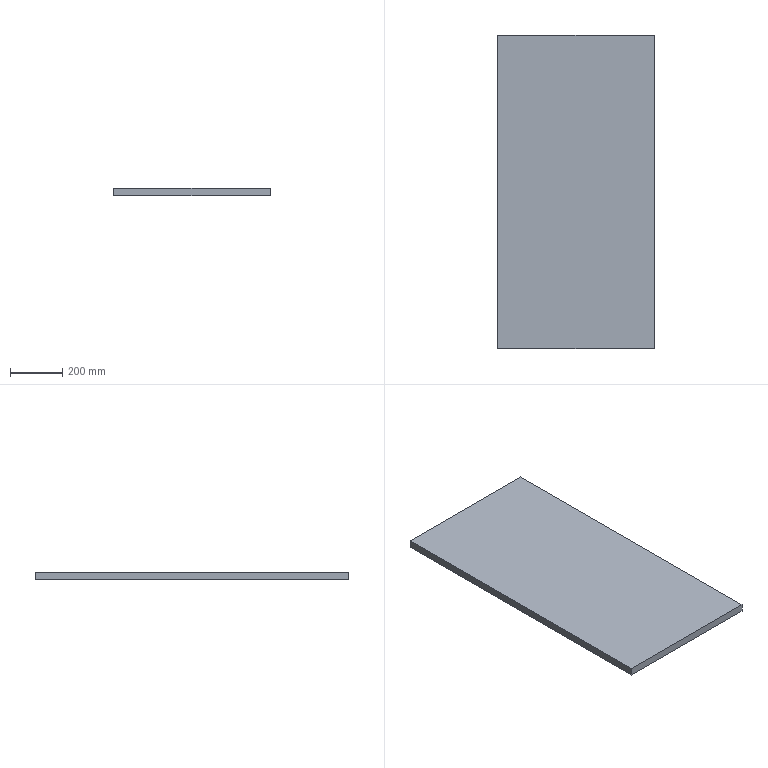Part | SolidWorks | features Extrusion 1, ICE 1 | 1 solid | 18 faces | box 600 x 1200 x 30 mm | volume 21509522 mm3 | plane 10 | cylinder 8 | commonest cylinder face diameters 120 x8
STEP:
#1=CARTESIAN_POINT('',(240.,-480.,2.));
#2=VERTEX_POINT('',#1);
#3=CARTESIAN_POINT('',(120.,-480.,2.));
#4=VERTEX_POINT('',#3);
#5=CARTESIAN_POINT('',(180.,-480.,2.));
#6=DIRECTION('',(0.,0.,-1.));
#7=DIRECTION('',(1.,0.,0.));
#8=AXIS2_PLACEMENT_3D('',#5,#6,#7);
#9=CIRCLE('',#8,60.);
#10=EDGE_CURVE('',#2,#4,#9,.T.);
#11=ORIENTED_EDGE('',*,*,#10,.F.);
#12=CARTESIAN_POINT('',(240.,-480.,0.));
#13=VERTEX_POINT('',#12);
#14=CARTESIAN_POINT('',(240.,-480.,2.));
#15=DIRECTION('',(0.,0.,-1.));
#16=VECTOR('',#15,1000.);
#17=LINE('',#14,#16);
#18=EDGE_CURVE('',#2,#13,#17,.T.);
#19=ORIENTED_EDGE('',*,*,#18,.T.);
#20=CARTESIAN_POINT('',(120.,-480.,0.));
#21=VERTEX_POINT('',#20);
#22=CARTESIAN_POINT('',(180.,-480.,0.));
#23=DIRECTION('',(0.,0.,-1.));
#24=DIRECTION('',(1.,0.,0.));
#25=AXIS2_PLACEMENT_3D('',#22,#23,#24);
#26=CIRCLE('',#25,60.);
#27=EDGE_CURVE('',#13,#21,#26,.T.);
#28=ORIENTED_EDGE('',*,*,#27,.T.);
#29=CARTESIAN_POINT('',(120.,-480.,2.));
#30=DIRECTION('',(0.,0.,-1.));
#31=VECTOR('',#30,1000.);
#32=LINE('',#29,#31);
#33=EDGE_CURVE('',#4,#21,#32,.T.);
#34=ORIENTED_EDGE('',*,*,#33,.F.);
#35=EDGE_LOOP('',(#11,#19,#28,#34));
#36=FACE_OUTER_BOUND('',#35,.T.);
#37=CARTESIAN_POINT('',(180.,-480.,2.));
#38=DIRECTION('',(0.,0.,-1.));
#39=DIRECTION('',(-1.,0.,0.));
#40=AXIS2_PLACEMENT_3D('',#37,#38,#39);
#41=CYLINDRICAL_SURFACE('',#40,60.);
#42=ADVANCED_FACE('',(#36),#41,.F.);
#43=CARTESIAN_POINT('',(-120.,-480.,2.));
#44=VERTEX_POINT('',#43);
#45=CARTESIAN_POINT('',(-240.,-480.,2.));
#46=VERTEX_POINT('',#45);
#47=CARTESIAN_POINT('',(-180.,-480.,2.));
#48=DIRECTION('',(0.,0.,-1.));
#49=DIRECTION('',(-1.,0.,0.));
#50=AXIS2_PLACEMENT_3D('',#47,#48,#49);
#51=CIRCLE('',#50,60.);
#52=EDGE_CURVE('',#44,#46,#51,.T.);
#53=ORIENTED_EDGE('',*,*,#52,.F.);
#54=CARTESIAN_POINT('',(-120.,-480.,0.));
#55=VERTEX_POINT('',#54);
#56=CARTESIAN_POINT('',(-120.,-480.,2.));
#57=DIRECTION('',(0.,0.,-1.));
#58=VECTOR('',#57,1000.);
#59=LINE('',#56,#58);
#60=EDGE_CURVE('',#44,#55,#59,.T.);
#61=ORIENTED_EDGE('',*,*,#60,.T.);
#62=CARTESIAN_POINT('',(-240.,-480.,0.));
#63=VERTEX_POINT('',#62);
#64=CARTESIAN_POINT('',(-180.,-480.,0.));
#65=DIRECTION('',(0.,0.,-1.));
#66=DIRECTION('',(-1.,0.,0.));
#67=AXIS2_PLACEMENT_3D('',#64,#65,#66);
#68=CIRCLE('',#67,60.);
#69=EDGE_CURVE('',#55,#63,#68,.T.);
#70=ORIENTED_EDGE('',*,*,#69,.T.);
#71=CARTESIAN_POINT('',(-240.,-480.,2.));
#72=DIRECTION('',(0.,0.,-1.));
#73=VECTOR('',#72,1000.);
#74=LINE('',#71,#73);
#75=EDGE_CURVE('',#46,#63,#74,.T.);
#76=ORIENTED_EDGE('',*,*,#75,.F.);
#77=EDGE_LOOP('',(#53,#61,#70,#76));
#78=FACE_OUTER_BOUND('',#77,.T.);
#79=CARTESIAN_POINT('',(-180.,-480.,2.));
#80=DIRECTION('',(0.,0.,-1.));
#81=DIRECTION('',(-1.,0.,0.));
#82=AXIS2_PLACEMENT_3D('',#79,#80,#81);
#83=CYLINDRICAL_SURFACE('',#82,60.);
#84=ADVANCED_FACE('',(#78),#83,.F.);
#85=CARTESIAN_POINT('',(-120.,480.,2.));
#86=VERTEX_POINT('',#85);
#87=CARTESIAN_POINT('',(-240.,480.,2.));
#88=VERTEX_POINT('',#87);
#89=CARTESIAN_POINT('',(-180.,480.,2.));
#90=DIRECTION('',(0.,0.,-1.));
#91=DIRECTION('',(1.,0.,0.));
#92=AXIS2_PLACEMENT_3D('',#89,#90,#91);
#93=CIRCLE('',#92,60.);
#94=EDGE_CURVE('',#86,#88,#93,.T.);
#95=ORIENTED_EDGE('',*,*,#94,.F.);
#96=CARTESIAN_POINT('',(-120.,480.,0.));
#97=VERTEX_POINT('',#96);
#98=CARTESIAN_POINT('',(-120.,480.,2.));
#99=DIRECTION('',(0.,0.,-1.));
#100=VECTOR('',#99,1000.);
#101=LINE('',#98,#100);
#102=EDGE_CURVE('',#86,#97,#101,.T.);
#103=ORIENTED_EDGE('',*,*,#102,.T.);
#104=CARTESIAN_POINT('',(-240.,480.,0.));
#105=VERTEX_POINT('',#104);
#106=CARTESIAN_POINT('',(-180.,480.,0.));
#107=DIRECTION('',(0.,0.,-1.));
#108=DIRECTION('',(1.,0.,0.));
#109=AXIS2_PLACEMENT_3D('',#106,#107,#108);
#110=CIRCLE('',#109,60.);
#111=EDGE_CURVE('',#97,#105,#110,.T.);
#112=ORIENTED_EDGE('',*,*,#111,.T.);
#113=CARTESIAN_POINT('',(-240.,480.,2.));
#114=DIRECTION('',(0.,0.,-1.));
#115=VECTOR('',#114,1000.);
#116=LINE('',#113,#115);
#117=EDGE_CURVE('',#88,#105,#116,.T.);
#118=ORIENTED_EDGE('',*,*,#117,.F.);
#119=EDGE_LOOP('',(#95,#103,#112,#118));
#120=FACE_OUTER_BOUND('',#119,.T.);
#121=CARTESIAN_POINT('',(-180.,480.,2.));
#122=DIRECTION('',(0.,0.,-1.));
#123=DIRECTION('',(-1.,0.,0.));
#124=AXIS2_PLACEMENT_3D('',#121,#122,#123);
#125=CYLINDRICAL_SURFACE('',#124,60.);
#126=ADVANCED_FACE('',(#120),#125,.F.);
#127=CARTESIAN_POINT('',(240.,480.,2.));
#128=VERTEX_POINT('',#127);
#129=CARTESIAN_POINT('',(120.,480.,2.));
#130=VERTEX_POINT('',#129);
#131=CARTESIAN_POINT('',(180.,480.,2.));
#132=DIRECTION('',(0.,0.,-1.));
#133=DIRECTION('',(-1.,0.,0.));
#134=AXIS2_PLACEMENT_3D('',#131,#132,#133);
#135=CIRCLE('',#134,60.);
#136=EDGE_CURVE('',#128,#130,#135,.T.);
#137=ORIENTED_EDGE('',*,*,#136,.F.);
#138=CARTESIAN_POINT('',(240.,480.,0.));
#139=VERTEX_POINT('',#138);
#140=CARTESIAN_POINT('',(240.,480.,2.));
#141=DIRECTION('',(0.,0.,-1.));
#142=VECTOR('',#141,1000.);
#143=LINE('',#140,#142);
#144=EDGE_CURVE('',#128,#139,#143,.T.);
#145=ORIENTED_EDGE('',*,*,#144,.T.);
#146=CARTESIAN_POINT('',(120.,480.,0.));
#147=VERTEX_POINT('',#146);
#148=CARTESIAN_POINT('',(180.,480.,0.));
#149=DIRECTION('',(0.,0.,-1.));
#150=DIRECTION('',(-1.,0.,0.));
#151=AXIS2_PLACEMENT_3D('',#148,#149,#150);
#152=CIRCLE('',#151,60.);
#153=EDGE_CURVE('',#139,#147,#152,.T.);
#154=ORIENTED_EDGE('',*,*,#153,.T.);
#155=CARTESIAN_POINT('',(120.,480.,2.));
#156=DIRECTION('',(0.,0.,-1.));
#157=VECTOR('',#156,1000.);
#158=LINE('',#155,#157);
#159=EDGE_CURVE('',#130,#147,#158,.T.);
#160=ORIENTED_EDGE('',*,*,#159,.F.);
#161=EDGE_LOOP('',(#137,#145,#154,#160));
#162=FACE_OUTER_BOUND('',#161,.T.);
#163=CARTESIAN_POINT('',(180.,480.,2.));
#164=DIRECTION('',(0.,0.,-1.));
#165=DIRECTION('',(-1.,0.,0.));
#166=AXIS2_PLACEMENT_3D('',#163,#164,#165);
#167=CYLINDRICAL_SURFACE('',#166,60.);
#168=ADVANCED_FACE('',(#162),#167,.F.);
#169=CARTESIAN_POINT('',(300.,-600.,0.));
#170=VERTEX_POINT('',#169);
#171=CARTESIAN_POINT('',(300.,600.,0.));
#172=VERTEX_POINT('',#171);
#173=CARTESIAN_POINT('',(300.,-600.,0.));
#174=DIRECTION('',(0.,1.,0.));
#175=VECTOR('',#174,1000.);
#176=LINE('',#173,#175);
#177=EDGE_CURVE('',#170,#172,#176,.T.);
#178=ORIENTED_EDGE('',*,*,#177,.T.);
#179=CARTESIAN_POINT('',(300.,600.,30.));
#180=VERTEX_POINT('',#179);
#181=CARTESIAN_POINT('',(300.,600.,30.));
#182=DIRECTION('',(0.,0.,-1.));
#183=VECTOR('',#182,1000.);
#184=LINE('',#181,#183);
#185=EDGE_CURVE('',#180,#172,#184,.T.);
#186=ORIENTED_EDGE('',*,*,#185,.F.);
#187=CARTESIAN_POINT('',(300.,-600.,30.));
#188=VERTEX_POINT('',#187);
#189=CARTESIAN_POINT('',(300.,-600.,30.));
#190=DIRECTION('',(0.,1.,0.));
#191=VECTOR('',#190,1000.);
#192=LINE('',#189,#191);
#193=EDGE_CURVE('',#188,#180,#192,.T.);
#194=ORIENTED_EDGE('',*,*,#193,.F.);
#195=CARTESIAN_POINT('',(300.,-600.,30.));
#196=DIRECTION('',(0.,0.,-1.));
#197=VECTOR('',#196,1000.);
#198=LINE('',#195,#197);
#199=EDGE_CURVE('',#188,#170,#198,.T.);
#200=ORIENTED_EDGE('',*,*,#199,.T.);
#201=EDGE_LOOP('',(#178,#186,#194,#200));
#202=FACE_OUTER_BOUND('',#201,.T.);
#203=CARTESIAN_POINT('',(300.,-600.,30.));
#204=DIRECTION('',(-1.,0.,0.));
#205=DIRECTION('',(0.,0.,1.));
#206=AXIS2_PLACEMENT_3D('',#203,#204,#205);
#207=PLANE('',#206);
#208=ADVANCED_FACE('',(#202),#207,.F.);
#209=CARTESIAN_POINT('',(-300.,600.,0.));
#210=VERTEX_POINT('',#209);
#211=CARTESIAN_POINT('',(-300.,600.,0.));
#212=DIRECTION('',(-1.,0.,0.));
#213=VECTOR('',#212,1000.);
#214=LINE('',#211,#213);
#215=EDGE_CURVE('',#172,#210,#214,.T.);
#216=ORIENTED_EDGE('',*,*,#215,.T.);
#217=CARTESIAN_POINT('',(-300.,600.,30.));
#218=VERTEX_POINT('',#217);
#219=CARTESIAN_POINT('',(-300.,600.,30.));
#220=DIRECTION('',(0.,0.,-1.));
#221=VECTOR('',#220,1000.);
#222=LINE('',#219,#221);
#223=EDGE_CURVE('',#218,#210,#222,.T.);
#224=ORIENTED_EDGE('',*,*,#223,.F.);
#225=CARTESIAN_POINT('',(-300.,600.,30.));
#226=DIRECTION('',(-1.,0.,0.));
#227=VECTOR('',#226,1000.);
#228=LINE('',#225,#227);
#229=EDGE_CURVE('',#180,#218,#228,.T.);
#230=ORIENTED_EDGE('',*,*,#229,.F.);
#231=ORIENTED_EDGE('',*,*,#185,.T.);
#232=EDGE_LOOP('',(#216,#224,#230,#231));
#233=FACE_OUTER_BOUND('',#232,.T.);
#234=CARTESIAN_POINT('',(-300.,600.,30.));
#235=DIRECTION('',(0.,-1.,0.));
#236=DIRECTION('',(0.,0.,-1.));
#237=AXIS2_PLACEMENT_3D('',#234,#235,#236);
#238=PLANE('',#237);
#239=ADVANCED_FACE('',(#233),#238,.F.);
#240=CARTESIAN_POINT('',(-300.,-600.,0.));
#241=VERTEX_POINT('',#240);
#242=CARTESIAN_POINT('',(-300.,-600.,0.));
#243=DIRECTION('',(0.,-1.,0.));
#244=VECTOR('',#243,1000.);
#245=LINE('',#242,#244);
#246=EDGE_CURVE('',#210,#241,#245,.T.);
#247=ORIENTED_EDGE('',*,*,#246,.T.);
#248=CARTESIAN_POINT('',(-300.,-600.,30.));
#249=VERTEX_POINT('',#248);
#250=CARTESIAN_POINT('',(-300.,-600.,30.));
#251=DIRECTION('',(0.,0.,-1.));
#252=VECTOR('',#251,1000.);
#253=LINE('',#250,#252);
#254=EDGE_CURVE('',#249,#241,#253,.T.);
#255=ORIENTED_EDGE('',*,*,#254,.F.);
#256=CARTESIAN_POINT('',(-300.,-600.,30.));
#257=DIRECTION('',(0.,-1.,0.));
#258=VECTOR('',#257,1000.);
#259=LINE('',#256,#258);
#260=EDGE_CURVE('',#218,#249,#259,.T.);
#261=ORIENTED_EDGE('',*,*,#260,.F.);
#262=ORIENTED_EDGE('',*,*,#223,.T.);
#263=EDGE_LOOP('',(#247,#255,#261,#262));
#264=FACE_OUTER_BOUND('',#263,.T.);
#265=CARTESIAN_POINT('',(-300.,-600.,30.));
#266=DIRECTION('',(1.,0.,0.));
#267=DIRECTION('',(0.,0.,-1.));
#268=AXIS2_PLACEMENT_3D('',#265,#266,#267);
#269=PLANE('',#268);
#270=ADVANCED_FACE('',(#264),#269,.F.);
#271=CARTESIAN_POINT('',(-300.,-600.,0.));
#272=DIRECTION('',(1.,0.,0.));
#273=VECTOR('',#272,1000.);
#274=LINE('',#271,#273);
#275=EDGE_CURVE('',#241,#170,#274,.T.);
#276=ORIENTED_EDGE('',*,*,#275,.T.);
#277=ORIENTED_EDGE('',*,*,#199,.F.);
#278=CARTESIAN_POINT('',(-300.,-600.,30.));
#279=DIRECTION('',(1.,0.,0.));
#280=VECTOR('',#279,1000.);
#281=LINE('',#278,#280);
#282=EDGE_CURVE('',#249,#188,#281,.T.);
#283=ORIENTED_EDGE('',*,*,#282,.F.);
#284=ORIENTED_EDGE('',*,*,#254,.T.);
#285=EDGE_LOOP('',(#276,#277,#283,#284));
#286=FACE_OUTER_BOUND('',#285,.T.);
#287=CARTESIAN_POINT('',(-300.,-600.,30.));
#288=DIRECTION('',(0.,1.,0.));
#289=DIRECTION('',(0.,0.,1.));
#290=AXIS2_PLACEMENT_3D('',#287,#288,#289);
#291=PLANE('',#290);
#292=ADVANCED_FACE('',(#286),#291,.F.);
#293=ORIENTED_EDGE('',*,*,#193,.T.);
#294=ORIENTED_EDGE('',*,*,#229,.T.);
#295=ORIENTED_EDGE('',*,*,#260,.T.);
#296=ORIENTED_EDGE('',*,*,#282,.T.);
#297=EDGE_LOOP('',(#293,#294,#295,#296));
#298=FACE_OUTER_BOUND('',#297,.T.);
#299=CARTESIAN_POINT('',(0.,0.,30.));
#300=DIRECTION('',(0.,0.,-1.));
#301=DIRECTION('',(-1.,0.,0.));
#302=AXIS2_PLACEMENT_3D('',#299,#300,#301);
#303=PLANE('',#302);
#304=ADVANCED_FACE('',(#298),#303,.F.);
#305=CARTESIAN_POINT('',(180.,-480.,0.));
#306=DIRECTION('',(0.,0.,-1.));
#307=DIRECTION('',(1.,0.,0.));
#308=AXIS2_PLACEMENT_3D('',#305,#306,#307);
#309=CIRCLE('',#308,60.);
#310=EDGE_CURVE('',#21,#13,#309,.T.);
#311=ORIENTED_EDGE('',*,*,#310,.F.);
#312=ORIENTED_EDGE('',*,*,#27,.F.);
#313=EDGE_LOOP('',(#311,#312));
#314=FACE_BOUND('',#313,.T.);
#315=CARTESIAN_POINT('',(-180.,-480.,0.));
#316=DIRECTION('',(0.,0.,-1.));
#317=DIRECTION('',(-1.,0.,0.));
#318=AXIS2_PLACEMENT_3D('',#315,#316,#317);
#319=CIRCLE('',#318,60.);
#320=EDGE_CURVE('',#63,#55,#319,.T.);
#321=ORIENTED_EDGE('',*,*,#320,.F.);
#322=ORIENTED_EDGE('',*,*,#69,.F.);
#323=EDGE_LOOP('',(#321,#322));
#324=FACE_BOUND('',#323,.T.);
#325=CARTESIAN_POINT('',(-180.,480.,0.));
#326=DIRECTION('',(0.,0.,-1.));
#327=DIRECTION('',(1.,0.,0.));
#328=AXIS2_PLACEMENT_3D('',#325,#326,#327);
#329=CIRCLE('',#328,60.);
#330=EDGE_CURVE('',#105,#97,#329,.T.);
#331=ORIENTED_EDGE('',*,*,#330,.F.);
#332=ORIENTED_EDGE('',*,*,#111,.F.);
#333=EDGE_LOOP('',(#331,#332));
#334=FACE_BOUND('',#333,.T.);
#335=CARTESIAN_POINT('',(180.,480.,0.));
#336=DIRECTION('',(0.,0.,-1.));
#337=DIRECTION('',(-1.,0.,0.));
#338=AXIS2_PLACEMENT_3D('',#335,#336,#337);
#339=CIRCLE('',#338,60.);
#340=EDGE_CURVE('',#147,#139,#339,.T.);
#341=ORIENTED_EDGE('',*,*,#340,.F.);
#342=ORIENTED_EDGE('',*,*,#153,.F.);
#343=EDGE_LOOP('',(#341,#342));
#344=FACE_BOUND('',#343,.T.);
#345=ORIENTED_EDGE('',*,*,#177,.F.);
#346=ORIENTED_EDGE('',*,*,#275,.F.);
#347=ORIENTED_EDGE('',*,*,#246,.F.);
#348=ORIENTED_EDGE('',*,*,#215,.F.);
#349=EDGE_LOOP('',(#345,#346,#347,#348));
#350=FACE_OUTER_BOUND('',#349,.T.);
#351=CARTESIAN_POINT('',(0.,0.,0.));
#352=DIRECTION('',(0.,0.,-1.));
#353=DIRECTION('',(-1.,0.,0.));
#354=AXIS2_PLACEMENT_3D('',#351,#352,#353);
#355=PLANE('',#354);
#356=ADVANCED_FACE('',(#314,#324,#334,#344,#350),#355,.T.);
#357=ORIENTED_EDGE('',*,*,#144,.F.);
#358=CARTESIAN_POINT('',(180.,480.,2.));
#359=DIRECTION('',(0.,0.,-1.));
#360=DIRECTION('',(-1.,0.,0.));
#361=AXIS2_PLACEMENT_3D('',#358,#359,#360);
#362=CIRCLE('',#361,60.);
#363=EDGE_CURVE('',#130,#128,#362,.T.);
#364=ORIENTED_EDGE('',*,*,#363,.F.);
#365=ORIENTED_EDGE('',*,*,#159,.T.);
#366=ORIENTED_EDGE('',*,*,#340,.T.);
#367=EDGE_LOOP('',(#357,#364,#365,#366));
#368=FACE_OUTER_BOUND('',#367,.T.);
#369=CARTESIAN_POINT('',(180.,480.,2.));
#370=DIRECTION('',(0.,0.,-1.));
#371=DIRECTION('',(-1.,0.,0.));
#372=AXIS2_PLACEMENT_3D('',#369,#370,#371);
#373=CYLINDRICAL_SURFACE('',#372,60.);
#374=ADVANCED_FACE('',(#368),#373,.F.);
#375=ORIENTED_EDGE('',*,*,#363,.T.);
#376=ORIENTED_EDGE('',*,*,#136,.T.);
#377=EDGE_LOOP('',(#375,#376));
#378=FACE_OUTER_BOUND('',#377,.T.);
#379=CARTESIAN_POINT('',(180.,480.,2.));
#380=DIRECTION('',(0.,0.,-1.));
#381=DIRECTION('',(-1.,0.,0.));
#382=AXIS2_PLACEMENT_3D('',#379,#380,#381);
#383=PLANE('',#382);
#384=ADVANCED_FACE('',(#378),#383,.T.);
#385=ORIENTED_EDGE('',*,*,#102,.F.);
#386=CARTESIAN_POINT('',(-180.,480.,2.));
#387=DIRECTION('',(0.,0.,-1.));
#388=DIRECTION('',(1.,0.,0.));
#389=AXIS2_PLACEMENT_3D('',#386,#387,#388);
#390=CIRCLE('',#389,60.);
#391=EDGE_CURVE('',#88,#86,#390,.T.);
#392=ORIENTED_EDGE('',*,*,#391,.F.);
#393=ORIENTED_EDGE('',*,*,#117,.T.);
#394=ORIENTED_EDGE('',*,*,#330,.T.);
#395=EDGE_LOOP('',(#385,#392,#393,#394));
#396=FACE_OUTER_BOUND('',#395,.T.);
#397=CARTESIAN_POINT('',(-180.,480.,2.));
#398=DIRECTION('',(0.,0.,-1.));
#399=DIRECTION('',(-1.,0.,0.));
#400=AXIS2_PLACEMENT_3D('',#397,#398,#399);
#401=CYLINDRICAL_SURFACE('',#400,60.);
#402=ADVANCED_FACE('',(#396),#401,.F.);
#403=ORIENTED_EDGE('',*,*,#391,.T.);
#404=ORIENTED_EDGE('',*,*,#94,.T.);
#405=EDGE_LOOP('',(#403,#404));
#406=FACE_OUTER_BOUND('',#405,.T.);
#407=CARTESIAN_POINT('',(-180.,480.,2.));
#408=DIRECTION('',(0.,0.,1.));
#409=DIRECTION('',(1.,0.,0.));
#410=AXIS2_PLACEMENT_3D('',#407,#408,#409);
#411=PLANE('',#410);
#412=ADVANCED_FACE('',(#406),#411,.F.);
#413=ORIENTED_EDGE('',*,*,#60,.F.);
#414=CARTESIAN_POINT('',(-180.,-480.,2.));
#415=DIRECTION('',(0.,0.,-1.));
#416=DIRECTION('',(-1.,0.,0.));
#417=AXIS2_PLACEMENT_3D('',#414,#415,#416);
#418=CIRCLE('',#417,60.);
#419=EDGE_CURVE('',#46,#44,#418,.T.);
#420=ORIENTED_EDGE('',*,*,#419,.F.);
#421=ORIENTED_EDGE('',*,*,#75,.T.);
#422=ORIENTED_EDGE('',*,*,#320,.T.);
#423=EDGE_LOOP('',(#413,#420,#421,#422));
#424=FACE_OUTER_BOUND('',#423,.T.);
#425=CARTESIAN_POINT('',(-180.,-480.,2.));
#426=DIRECTION('',(0.,0.,-1.));
#427=DIRECTION('',(-1.,0.,0.));
#428=AXIS2_PLACEMENT_3D('',#425,#426,#427);
#429=CYLINDRICAL_SURFACE('',#428,60.);
#430=ADVANCED_FACE('',(#424),#429,.F.);
#431=ORIENTED_EDGE('',*,*,#419,.T.);
#432=ORIENTED_EDGE('',*,*,#52,.T.);
#433=EDGE_LOOP('',(#431,#432));
#434=FACE_OUTER_BOUND('',#433,.T.);
#435=CARTESIAN_POINT('',(-180.,-480.,2.));
#436=DIRECTION('',(0.,0.,-1.));
#437=DIRECTION('',(-1.,0.,0.));
#438=AXIS2_PLACEMENT_3D('',#435,#436,#437);
#439=PLANE('',#438);
#440=ADVANCED_FACE('',(#434),#439,.T.);
#441=ORIENTED_EDGE('',*,*,#18,.F.);
#442=CARTESIAN_POINT('',(180.,-480.,2.));
#443=DIRECTION('',(0.,0.,-1.));
#444=DIRECTION('',(1.,0.,0.));
#445=AXIS2_PLACEMENT_3D('',#442,#443,#444);
#446=CIRCLE('',#445,60.);
#447=EDGE_CURVE('',#4,#2,#446,.T.);
#448=ORIENTED_EDGE('',*,*,#447,.F.);
#449=ORIENTED_EDGE('',*,*,#33,.T.);
#450=ORIENTED_EDGE('',*,*,#310,.T.);
#451=EDGE_LOOP('',(#441,#448,#449,#450));
#452=FACE_OUTER_BOUND('',#451,.T.);
#453=CARTESIAN_POINT('',(180.,-480.,2.));
#454=DIRECTION('',(0.,0.,-1.));
#455=DIRECTION('',(-1.,0.,0.));
#456=AXIS2_PLACEMENT_3D('',#453,#454,#455);
#457=CYLINDRICAL_SURFACE('',#456,60.);
#458=ADVANCED_FACE('',(#452),#457,.F.);
#459=ORIENTED_EDGE('',*,*,#447,.T.);
#460=ORIENTED_EDGE('',*,*,#10,.T.);
#461=EDGE_LOOP('',(#459,#460));
#462=FACE_OUTER_BOUND('',#461,.T.);
#463=CARTESIAN_POINT('',(180.,-480.,2.));
#464=DIRECTION('',(0.,0.,1.));
#465=DIRECTION('',(1.,0.,0.));
#466=AXIS2_PLACEMENT_3D('',#463,#464,#465);
#467=PLANE('',#466);
#468=ADVANCED_FACE('',(#462),#467,.F.);
#469=CLOSED_SHELL('',(#42,#84,#126,#168,#208,#239,#270,#292,#304,#356,#374,#384,#402,#412,#430,#440,#458,#468));
#470=MANIFOLD_SOLID_BREP('',#469);
#471=CARTESIAN_POINT('',(0.,0.,0.));
#472=DIRECTION('',(0.,0.,1.));
#473=DIRECTION('',(1.,0.,0.));
#474=AXIS2_PLACEMENT_3D('',#471,#472,#473);
#475=(LENGTH_UNIT()NAMED_UNIT(*)SI_UNIT(.MILLI.,.METRE.));
#476=UNCERTAINTY_MEASURE_WITH_UNIT(LENGTH_MEASURE(0.00001),#475,'','');
#477=(NAMED_UNIT(*)PLANE_ANGLE_UNIT()SI_UNIT($,.RADIAN.));
#478=(NAMED_UNIT(*)SI_UNIT($,.STERADIAN.)SOLID_ANGLE_UNIT());
#479=(GEOMETRIC_REPRESENTATION_CONTEXT(3)GLOBAL_UNCERTAINTY_ASSIGNED_CONTEXT((#476))GLOBAL_UNIT_ASSIGNED_CONTEXT((#475,#477,#478))REPRESENTATION_CONTEXT('',''));
#480=ADVANCED_BREP_SHAPE_REPRESENTATION('',(#470,#474),#479);